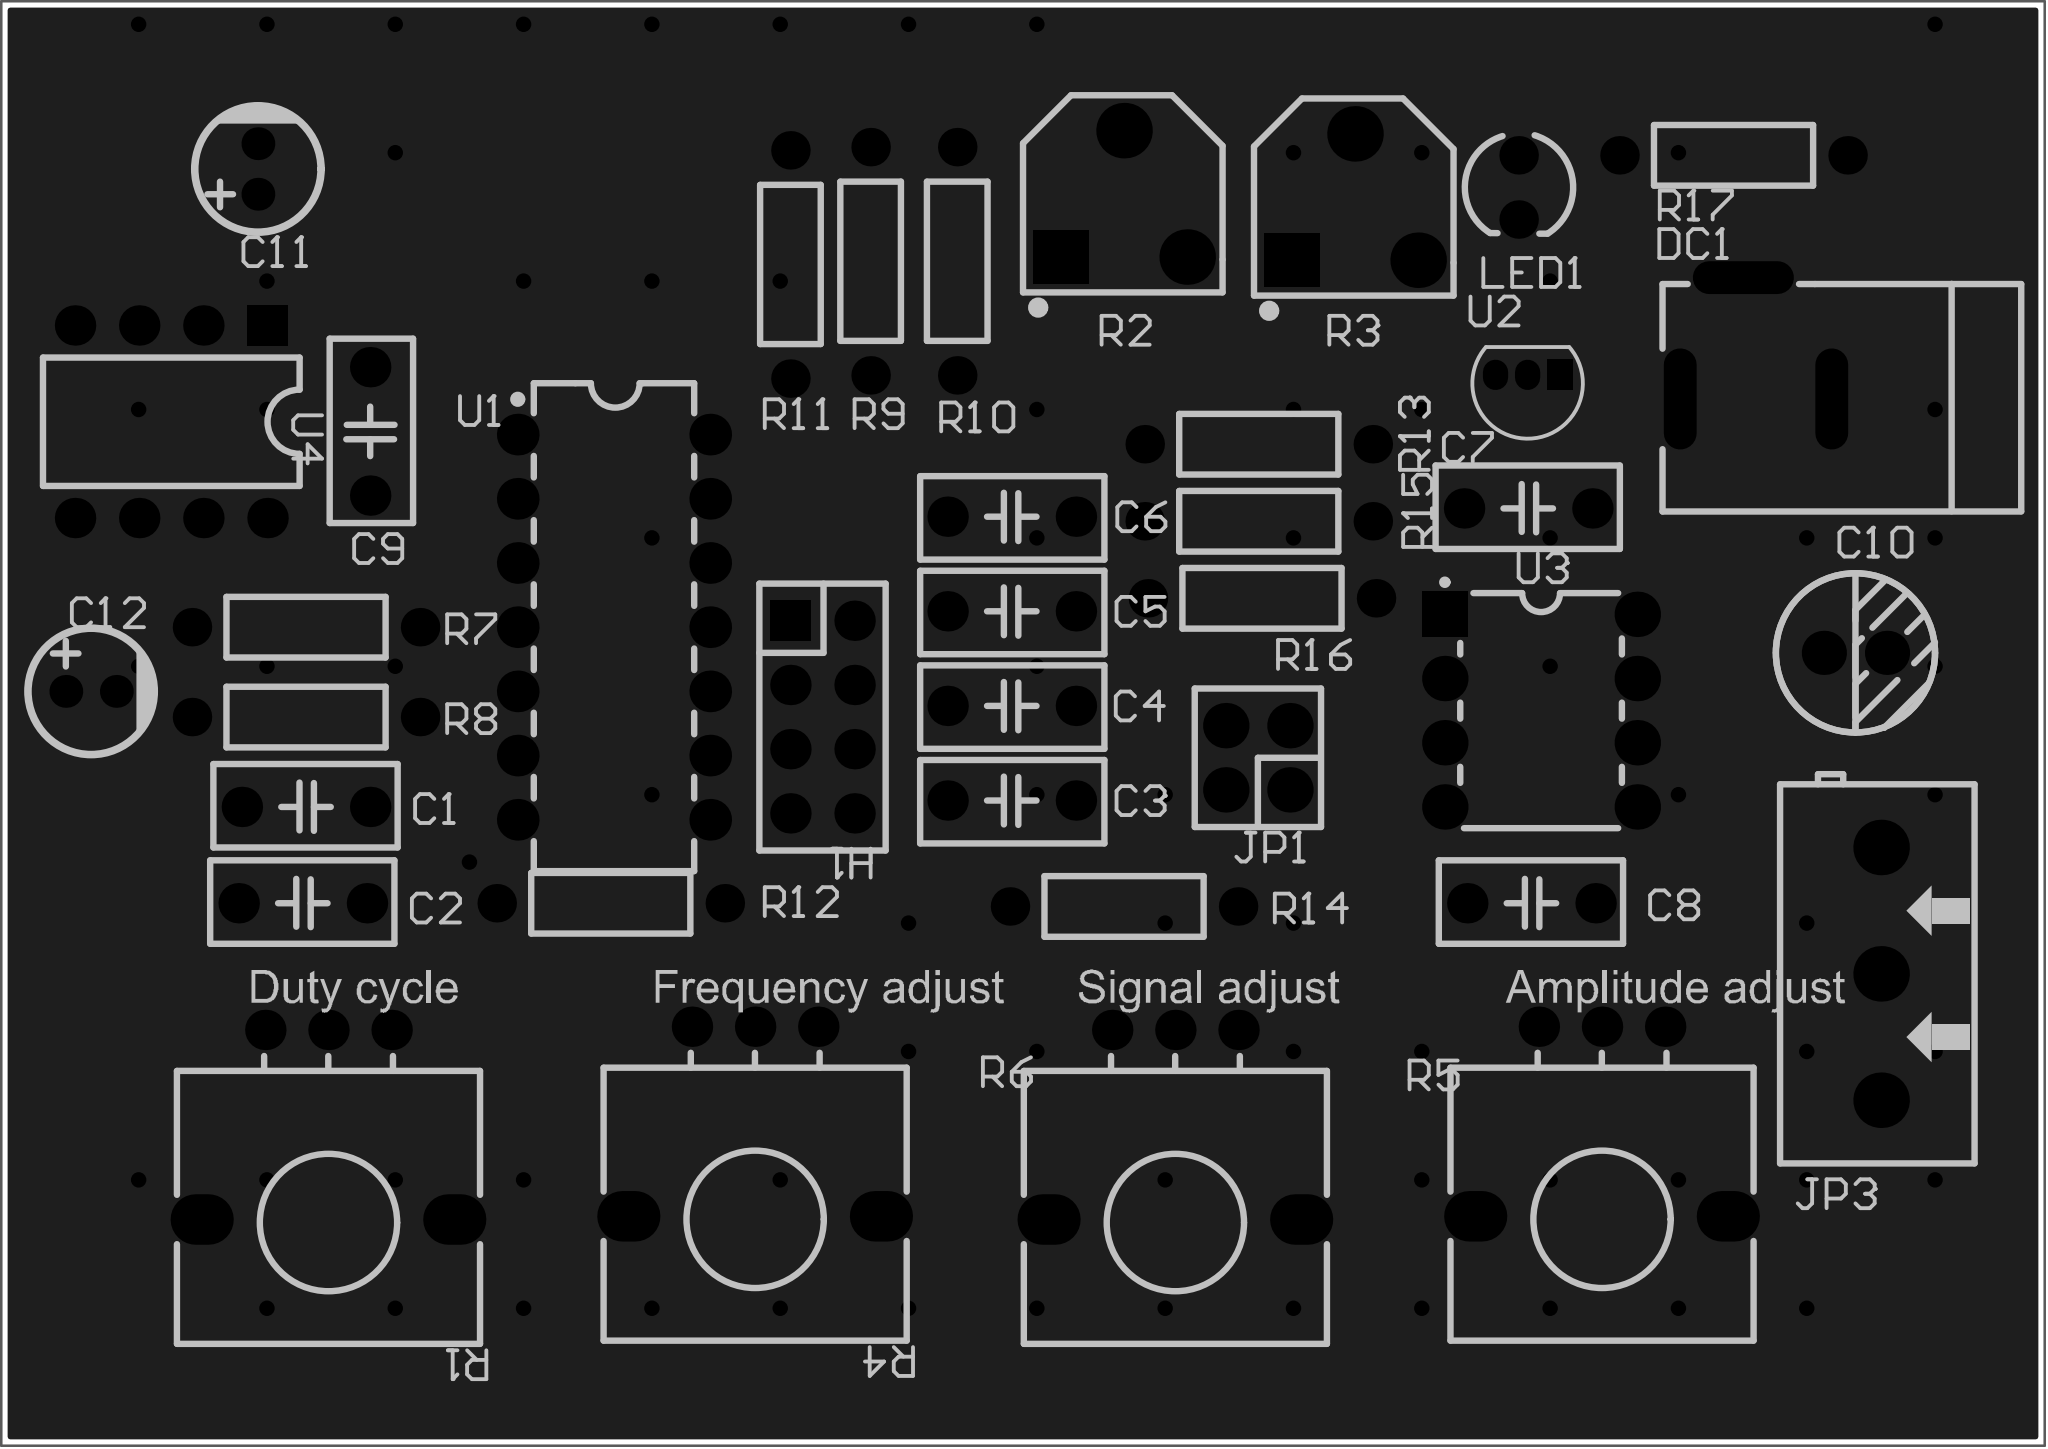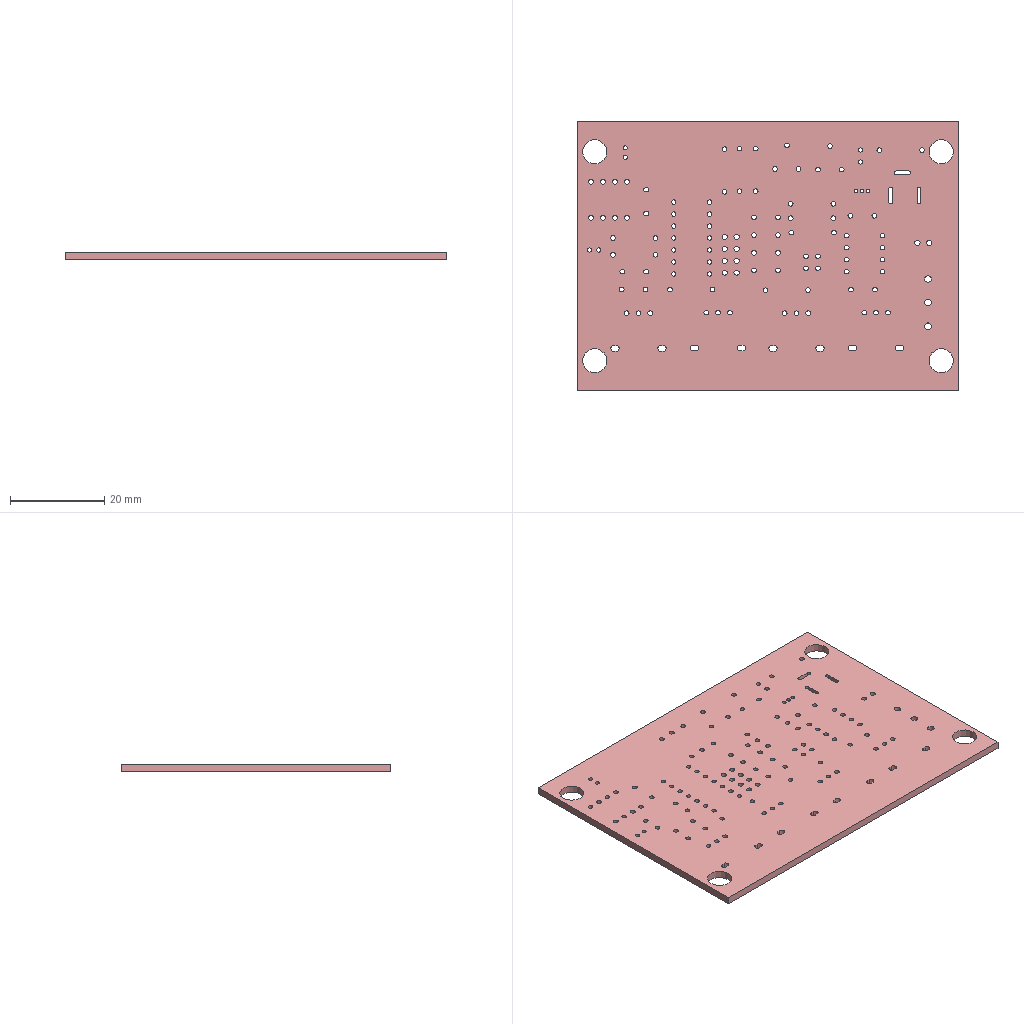Circuit board layout | Altium Designer | box 80.9 x 57.1 x 1.6 mm
Layer stack:
# Altium Designer layer stack of  (unit mm; dielectric type: 0 none, 1 core, 2 prepreg, 3 surface material)
index,name,kind,layer,copper_thickness_mm,dielectric_type,dielectric_thickness_mm,dielectric_material,dielectric_constant
0,Top Paste Mask Layer,other,,,,,,
1,Top Silkscreen Layer,other,,,,,,
2,Top Solder Mask Layer,dielectric,,,3,0.01,,3.3
3,Top Layer,copper,Top Layer,0.035,,,,
4,Dielectric1,dielectric,,,3,1.51,FR4,4.5
5,Bottom Layer,copper,Bottom Layer,0.035,,,,
6,Bottom Solder Mask Layer,dielectric,,,3,0.01,,3.3
7,Bottom Silkscreen Layer,other,,,,,,
8,Bottom Paste Mask Layer,other,,,,,,
# drill layer pairs: low layer,high layer
drill_pair,Top Layer,Bottom Layer
Part placement:
Designator,Comment,Layer,Footprint,Center-X(mm),Center-Y(mm),Rotation
C12,10uF,TopLayer,CAP-TH_BD5.0-P2.00-D0.8-FD-10UF50VC110GL,86.741,115.443,0
U4,TC7660S,TopLayer,DIP-8_L10.0-W6.5-P2.54-LS7.6-BL,89.916,126.111,180
R7,1kΩ,TopLayer,Res_1/4W,95.25,117.983,0
R8,10kΩ,TopLayer,Res_1/4W,95.25,114.427,0
R1,10kΩ,TopLayer,RES-ADJ-TH_R09512N0-FB15A7.0-B103-005,96.139,98.298,180
C2,100nF,TopLayer,CAP-TH_L5.1-W3.2-P5.08-D0.50,95.123,107.061,0
C1,100nF,TopLayer,CAP-TH_L5.1-W3.2-P5.08-D0.50,95.25,110.871,0
C11,10uF,TopLayer,CAP-TH_BD5.0-P2.00-D0.8-FD-10UF50VC110GL,93.345,136.112,90
C9,100nF,TopLayer,CAP-TH_L5.1-W3.2-P5.08-D0.50,97.79,125.73,270
R12,30kΩ,TopLayer,Res_1/4W,107.315,107.061,0
U1,ICL8038CCPD,TopLayer,PDIP-14_L19.2-W6.6-P2.54-LS7.6-BL,107.442,117.983,270
R4,10kΩ,TopLayer,RES-ADJ-TH_R09512N0-FB15A7.0-B103-005,113.03,98.425,180
H1,,TopLayer,HDR-TH_8P-P2.54-V-F-R2-C4-S2.54-1,115.697,114.427,270
R11,4.7kΩ,TopLayer,Res_1/4W,114.427,132.334,90
R9,10kΩ,TopLayer,Res_1/4W,117.602,132.461,270
C6,101,TopLayer,CAP-TH_L5.1-W3.2-P5.08-D0.50,123.19,122.355,180
C5,101,TopLayer,CAP-TH_L5.1-W3.2-P5.08-D0.50,123.19,118.612,180
C3,101,TopLayer,CAP-TH_L5.1-W3.2-P5.08-D0.50,123.19,111.125,180
C4,101,TopLayer,CAP-TH_L5.1-W3.2-P5.08-D0.50,123.19,114.868,180
R10,10kΩ,TopLayer,Res_1/4W,121.031,132.461,90
R14,4.7kΩ,TopLayer,Res_1/4W,127.635,106.934,0
R6,10kΩ,TopLayer,RES-ADJ-TH_R09512N0-FB15A7.0-B103-005,129.667,98.298,180
R2,100kΩ,TopLayer,RES-ADJ-SMD_RM065-V1,127.635,135.128,0
R15,10kΩ,TopLayer,Res_1/4W,132.969,122.174,0
R13,10kΩ,TopLayer,Res_1/4W,132.969,125.222,180
R16,10kΩ,TopLayer,Res_1/4W,133.096,119.126,0
JP1,,TopLayer,HDR-TH_4P-P2.54-V-F-R2-C2-S2.54,132.934,112.816,90
R3,100kΩ,TopLayer,RES-ADJ-SMD_RM065-V1,136.779,135.001,0
U3,,TopLayer,DIP-8_L9.3-W6.4-P2.54-LS7.6-TL,144.145,114.681,0
C7,100nF,TopLayer,CAP-TH_L5.1-W3.2-P5.08-D0.50,143.637,122.682,0
C8,100nF,TopLayer,CAP-TH_L5.1-W3.2-P5.08-D0.50,143.764,107.061,0
R5,10kΩ,TopLayer,RES-ADJ-TH_R09512N0-FB15A7.0-B103-005,146.558,98.425,180
U2,78l09,TopLayer,TO-92-3_L4.5-W3.5-P1.27-L,143.612,127.966,180
LED1,,TopLayer,LED_TH-3mm,143.256,135.382,270
R17,10kΩ,TopLayer,Res_1/4W,151.765,136.652,0
DC1,,TopLayer,DC-2.0,152.654,129.413,0
C10,100uF,TopLayer,CAP-TH_BD6.3-P2.5-D0.6-FD-RYHG35V100UF,156.591,116.967,0
JP3,,TopLayer,CONN-TH_3P-P5.00_KF301-5.0-3P,157.607,104.267,90
Pad and via stacks:
# Altium Designer via and pad stacks of  (unit mm). Each distinct definition once, with the count of objects using it.
# via: kind,start_layer,end_layer,hole_mm,diameter_mm,mode(0 simple;1 top-mid-bottom;2 full stack),diameter_per_layer,count,example_net
# pad: kind,layer,hole_mm,hole_type(0 round;1 square;2 slot),plating,top_size,top_shape(1 round;2 rect;3 octagon;9 rounded rect),mid_size,bottom_size,mode,footprint,size_per_layer,count,example
pad,Multi-Layer,0.9,0,plated,1.3x1.3,1,1.3x1.3,1.3x1.3,0,CAP-TH_BD5.0-P2.00-D0.8-FD-10UF50VC110GL,,4,C12.2
pad,Multi-Layer,1,0,plated,1.6x1.6,2,1.6x1.6,1.6x1.6,0,DIP-8_L10.0-W6.5-P2.54-LS7.6-BL,,1,U4.1
pad,Multi-Layer,1,0,plated,1.6x1.6,1,1.6x1.6,1.6x1.6,0,DIP-8_L10.0-W6.5-P2.54-LS7.6-BL,,7,U4.2
pad,Multi-Layer,1,0,plated,1.524x1.524,1,1.524x1.524,1.524x1.524,0,Res_1/4W,,22,R7.1
pad,Multi-Layer,1,0,plated,1.6x1.6,1,1.6x1.6,1.6x1.6,0,RES-ADJ-TH_R09512N0-FB15A7.0-B103-005,,12,R1.1
pad,Multi-Layer,1.2,2,plated,2.5x2,1,2.5x2,2.5x2,0,RES-ADJ-TH_R09512N0-FB15A7.0-B103-005,,8,R1.4
pad,Multi-Layer,1,0,plated,1.6x1.6,1,1.6x1.6,1.6x1.6,0,CAP-TH_L5.1-W3.2-P5.08-D0.50,,18,C2.2
pad,Multi-Layer,0.95,0,plated,1.65x1.65,1,1.65x1.65,1.65x1.65,0,PDIP-14_L19.2-W6.6-P2.54-LS7.6-BL,,14,U1.1
pad,Multi-Layer,1.1,0,plated,1.6x1.6,2,1.6x1.6,1.6x1.6,0,HDR-TH_8P-P2.54-V-F-R2-C4-S2.54-1,,1,H1.1
pad,Multi-Layer,1.1,0,plated,1.6x1.6,1,1.6x1.6,1.6x1.6,0,HDR-TH_8P-P2.54-V-F-R2-C4-S2.54-1,,7,H1.2
pad,Multi-Layer,1,0,plated,2.2x2.1,2,2.2x2.1,2.2x2.1,0,RES-ADJ-SMD_RM065-V1,,2,R2.1
pad,Multi-Layer,1,0,plated,2.2x2.2,1,2.2x2.2,2.2x2.2,0,RES-ADJ-SMD_RM065-V1,,4,R2.3
pad,Multi-Layer,1,0,plated,1.8x1.8,1,1.8x1.8,1.8x1.8,0,HDR-TH_4P-P2.54-V-F-R2-C2-S2.54,,4,JP1.4
pad,Multi-Layer,1,0,plated,1.8x1.8,2,1.8x1.8,1.8x1.8,0,DIP-8_L9.3-W6.4-P2.54-LS7.6-TL,,1,U3.1
pad,Multi-Layer,1,0,plated,1.8x1.8,1,1.8x1.8,1.8x1.8,0,DIP-8_L9.3-W6.4-P2.54-LS7.6-TL,,7,U3.2
pad,Multi-Layer,0.7,2,plated,1x1.2,2,1x1.2,1x1.2,0,TO-92-3_L4.5-W3.5-P1.27-L,,1,U2.1
pad,Multi-Layer,0.7,2,plated,1x1.2,1,1x1.2,1x1.2,0,TO-92-3_L4.5-W3.5-P1.27-L,,2,U2.2
pad,Multi-Layer,0.9144,0,plated,1.524x1.524,1,1.524x1.524,1.524x1.524,0,LED_TH-3mm,,2,LED1.1
pad,Multi-Layer,0.8001,2,plated,4x1.3,1,4x1.3,4x1.3,0,DC-2.0,,3,DC1.2
pad,Multi-Layer,1.1,0,plated,1.75x1.75,1,1.75x1.75,1.75x1.75,0,CAP-TH_BD6.3-P2.5-D0.6-FD-RYHG35V100UF,,2,C10.2
pad,Multi-Layer,1.4,0,plated,2.2x2.2,1,2.2x2.2,2.2x2.2,0,CONN-TH_3P-P5.00_KF301-5.0-3P,,3,JP3.1
via,Top Layer,Bottom Layer,0.3048,0.61,0,,76,GND
Copper pours:
name,layer,net,type(0 solid;1 hatched;2 none)
Top Layer-GND,Top Layer,GND,0
Bottom Layer-GND,Bottom Layer,GND,0
Design rules, without the lines most boards share:
# Altium Designer design rules of  (exported by Altium Designer, unit mm)
# columns: name | kind | enabled | priority | scope1 | scope2 | descriptor | typed fields (field=value)
creepage | 65 | enabled | 1 | All | All | Creepage Distance Constraint =(0mil) (All),(All) |